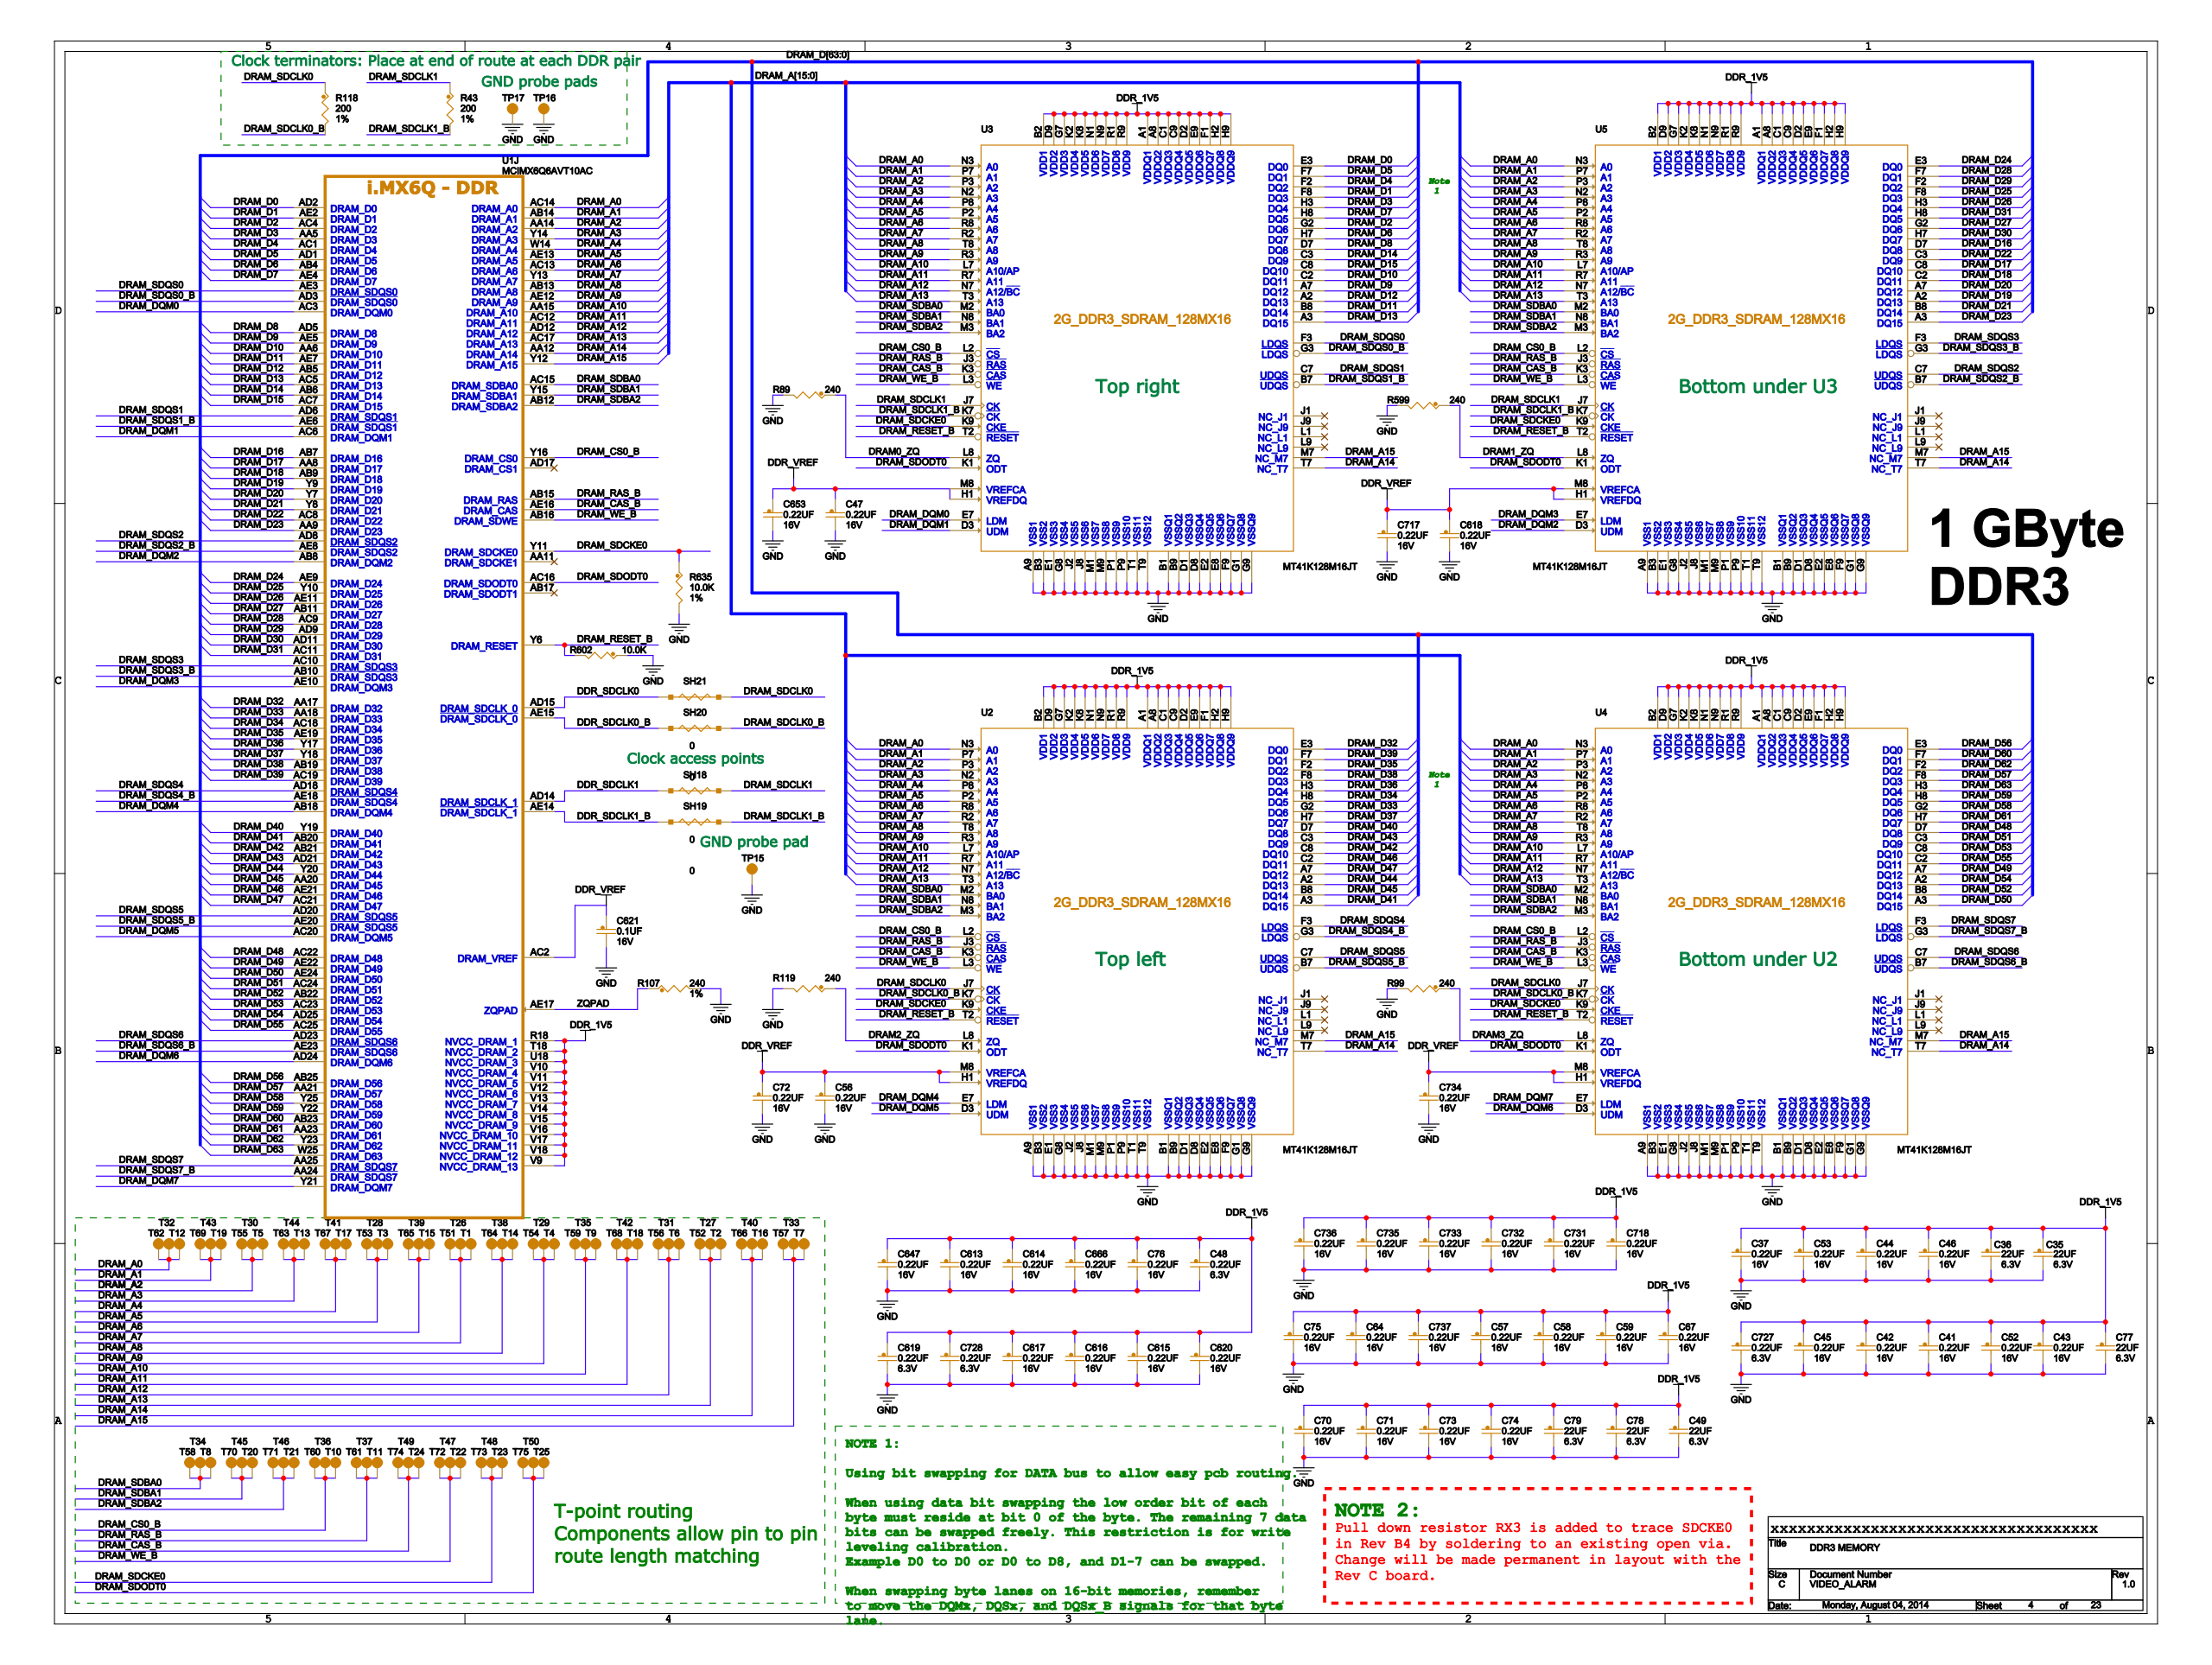Circuit board | Cadence Allegro | 994 parts | 728 nets | one sheet of the schematic
Parts on this sheet (reference | value | footprint):
C35 | 22UF | 0805_CC
C36 | 22UF | 0805_CC
C37 | 0.22UF | 0402_CC
C41 | 0.22UF | 0402_CC
C42 | 0.22UF | 0402_CC
C43 | 0.22UF | 0402_CC
C44 | 0.22UF | 0402_CC
C45 | 0.22UF | 0402_CC
C46 | 0.22UF | 0402_CC
C47 | 0.22UF | 0402_CC
C48 | 0.22UF | 0201_CC
C49 | 22UF | 0805_CC
C52 | 0.22UF | 0402_CC
C53 | 0.22UF | 0402_CC
C56 | 0.22UF | 0402_CC
C57 | 0.22UF | 0402_CC
C58 | 0.22UF | 0402_CC
C59 | 0.22UF | 0402_CC
C64 | 0.22UF | 0402_CC
C67 | 0.22UF | 0402_CC
C70 | 0.22UF | 0402_CC
C71 | 0.22UF | 0402_CC
C72 | 0.22UF | 0402_CC
C73 | 0.22UF | 0402_CC
C74 | 0.22UF | 0402_CC
C75 | 0.22UF | 0402_CC
C76 | 0.22UF | 0402_CC
C77 | 22UF | 0805_CC
C78 | 22UF | 0805_CC
C79 | 22UF | 0805_CC
C613 | 0.22UF | 0402_CC
C614 | 0.22UF | 0402_CC
C615 | 0.22UF | 0402_CC
C616 | 0.22UF | 0402_CC
C617 | 0.22UF | 0402_CC
C618 | 0.22UF | 0402_CC
C619 | 0.22UF | 0201_CC
C620 | 0.22UF | 0402_CC
C621 | 0.1UF | 0402_CC
C647 | 0.22UF | 0402_CC
C653 | 0.22UF | 0402_CC
C666 | 0.22UF | 0402_CC
C717 | 0.22UF | 0402_CC
C718 | 0.22UF | 0402_CC
C727 | 0.22UF | 0201_CC
C728 | 0.22UF | 0201_CC
C731 | 0.22UF | 0402_CC
C732 | 0.22UF | 0402_CC
C733 | 0.22UF | 0402_CC
C734 | 0.22UF | 0402_CC
C735 | 0.22UF | 0402_CC
C736 | 0.22UF | 0402_CC
C737 | 0.22UF | 0402_CC
J8 | 10029449-001RLF | HDMI
R43 | 200 | 0402_CC
R89 | 240 | 0402_CC
R99 | 240 | 0402_CC
R107 | 240 | 0402_CC
R118 | 200 | 0402_CC
R119 | 240 | 0402_CC
R599 | 240 | 0402_CC
R602 | 10.0K | 0402_CC
R635 | 10.0K | 0402_CC
SH18 | 0 | SH0201_CC
SH19 | 0 | SH0201_CC
SH20 | 0 | SH0201_CC
SH21 | 0 | SH0201_CC
T1 | TPAD_015 | TPAD_015
T2 | TPAD_015 | TPAD_015
T3 | TPAD_015 | TPAD_015
T4 | TPAD_015 | TPAD_015
T5 | TPAD_015 | TPAD_015
T6 | TPAD_015 | TPAD_015
T7 | TPAD_015 | TPAD_015
T8 | TPAD_015 | TPAD_015
T9 | TPAD_015 | TPAD_015
T10 | TPAD_015 | TPAD_015
T11 | TPAD_015 | TPAD_015
T12 | TPAD_015 | TPAD_015
T13 | TPAD_015 | TPAD_015
T14 | TPAD_015 | TPAD_015
T15 | TPAD_015 | TPAD_015
T16 | TPAD_015 | TPAD_015
T17 | TPAD_015 | TPAD_015
T18 | TPAD_015 | TPAD_015
T19 | TPAD_015 | TPAD_015
T20 | TPAD_015 | TPAD_015
T21 | TPAD_015 | TPAD_015
T22 | TPAD_015 | TPAD_015
T23 | TPAD_015 | TPAD_015
T24 | TPAD_015 | TPAD_015
T25 | TPAD_015 | TPAD_015
T26 | TPAD_015 | TPAD_015
T27 | TPAD_015 | TPAD_015
T28 | TPAD_015 | TPAD_015
T29 | TPAD_015 | TPAD_015
T30 | TPAD_015 | TPAD_015
T31 | TPAD_015 | TPAD_015
T32 | TPAD_015 | TPAD_015
T33 | TPAD_015 | TPAD_015
T34 | TPAD_015 | TPAD_015
T35 | TPAD_015 | TPAD_015
T36 | TPAD_015 | TPAD_015
T37 | TPAD_015 | TPAD_015
T38 | TPAD_015 | TPAD_015
T39 | TPAD_015 | TPAD_015
T40 | TPAD_015 | TPAD_015
T41 | TPAD_015 | TPAD_015
T42 | TPAD_015 | TPAD_015
T43 | TPAD_015 | TPAD_015
T44 | TPAD_015 | TPAD_015
T45 | TPAD_015 | TPAD_015
T46 | TPAD_015 | TPAD_015
T47 | TPAD_015 | TPAD_015
T48 | TPAD_015 | TPAD_015
T49 | TPAD_015 | TPAD_015
T50 | TPAD_015 | TPAD_015
T51 | TPAD_015 | TPAD_015
T52 | TPAD_015 | TPAD_015
T53 | TPAD_015 | TPAD_015
T54 | TPAD_015 | TPAD_015
T55 | TPAD_015 | TPAD_015
T56 | TPAD_015 | TPAD_015
T57 | TPAD_015 | TPAD_015
T58 | TPAD_015 | TPAD_015
T59 | TPAD_015 | TPAD_015
T60 | TPAD_015 | TPAD_015
T61 | TPAD_015 | TPAD_015
T62 | TPAD_015 | TPAD_015
T63 | TPAD_015 | TPAD_015
T64 | TPAD_015 | TPAD_015
T65 | TPAD_015 | TPAD_015
T66 | TPAD_015 | TPAD_015
T67 | TPAD_015 | TPAD_015
T68 | TPAD_015 | TPAD_015
T69 | TPAD_015 | TPAD_015
T70 | TPAD_015 | TPAD_015
T71 | TPAD_015 | TPAD_015
T72 | TPAD_015 | TPAD_015
T73 | TPAD_015 | TPAD_015
T74 | TPAD_015 | TPAD_015
T75 | TPAD_015 | TPAD_015
TP15 | TPAD_020 | TPAD_020
TP16 | TPAD_020 | TPAD_020
TP17 | TPAD_020 | TPAD_020
U1 | MCIMX6Q6AVT10AC | BGA624_0P8_21X21
U2 | MT41K128M16JT | BGA96_0P8_8P15X14P15
U3 | MT41K128M16JT | BGA96_0P8_8P15X14P15
U4 | MT41K128M16JT | BGA96_0P8_8P15X14P15
U5 | MT41K128M16JT | BGA96_0P8_8P15X14P15
Nets of these parts (net: part-pin ...):
GND: C35-2 C36-2 C37-2 C41-2 C42-2 C43-2 C44-2 C45-2 C46-2 C47-2 C48-2 C49-2 C52-2 C53-2 C56-2 C57-2 C58-2 C59-2 C64-2 C67-2 C70-2 C71-2 C72-2 C73-2 C74-2 C75-2 C76-2 C77-2 C78-2 C79-2 C613-2 C614-2 C615-2 C616-2 C617-2 C618-2 C619-2 C620-2 C621-2 C647-2 C653-2 C666-2 C717-2 C718-2 C727-2 C728-2 C731-2 C732-2 C733-2 C734-2 C735-2 C736-2 C737-2 R89-2 R99-2 R107-2 R119-2 R599-2 R602-1 R635-2 TP15-1 TP16-1 TP17-1 J8-2 J8-5 U1-A4 U1-A5 U1-A8 U1-A13 U1-B4 U1-C1 U1-D3 U1-D8 U1-E7 U1-F7 U1-F8 U1-G3 U1-H8 U1-J2 U1-J8 U1-K8 U1-L2 U1-L8 U1-M8 U1-N8 U1-P8 U1-R8 U1-T8 U1-T11 U1-T12 U1-T15 U1-T17 U1-T19 U2-A9 U2-B1 U2-B3 U2-B9 U2-D1 U2-D8 U2-E1 U2-E2 U2-E8 U2-F9 U2-G1 U2-G8 U2-G9 U2-J2 U2-J8 U2-M1 U2-M9 U2-P1 U2-P9 U2-T1 U2-T9 U3-A9 U3-B1 U3-B3 U3-B9 U3-D1 U3-D8 U3-E1 U3-E2 U3-E8 U3-F9 U3-G1 U3-G8 U3-G9 U3-J2 U3-J8 U3-M1 U3-M9 U3-P1 U3-P9 U3-T1 U3-T9 U4-A9 U4-B1 U4-B3 U4-B9 U4-D1 U4-D8 U4-E1 U4-E2 U4-E8 U4-F9 U4-G1 U4-G8 U4-G9 U4-J2 U4-J8 U4-M1 U4-M9 U4-P1 U4-P9 U4-T1 U4-T9 U5-A9 U5-B1 U5-B3 U5-B9 U5-D1 U5-D8 U5-E1 U5-E2 U5-E8 U5-F9 U5-G1 U5-G8 U5-G9 U5-J2 U5-J8 U5-M1 U5-M9 U5-P1 U5-P9 U5-T1 U5-T9
DDR_1V5: C35-1 C36-1 C37-1 C41-1 C42-1 C43-1 C44-1 C45-1 C46-1 C48-1 C49-1 C52-1 C53-1 C57-1 C58-1 C59-1 C64-1 C67-1 C70-1 C71-1 C73-1 C74-1 C75-1 C76-1 C77-1 C78-1 C79-1 C613-1 C614-1 C615-1 C616-1 C617-1 C619-1 C620-1 C647-1 C666-1 C718-1 C727-1 C728-1 C731-1 C732-1 C733-1 C735-1 C736-1 C737-1 U1-R18 U1-T18 U1-U18 U1-V9 U1-V10 U1-V11 U1-V12 U1-V13 U1-V14 U1-V15 U1-V16 U1-V17 U1-V18 U2-A1 U2-A8 U2-B2 U2-C1 U2-C9 U2-D2 U2-D9 U2-E9 U2-F1 U2-G7 U2-H2 U2-H9 U2-K2 U2-K8 U2-N1 U2-N9 U2-R1 U2-R9 U3-A1 U3-A8 U3-B2 U3-C1 U3-C9 U3-D2 U3-D9 U3-E9 U3-F1 U3-G7 U3-H2 U3-H9 U3-K2 U3-K8 U3-N1 U3-N9 U3-R1 U3-R9 U4-A1 U4-A8 U4-B2 U4-C1 U4-C9 U4-D2 U4-D9 U4-E9 U4-F1 U4-G7 U4-H2 U4-H9 U4-K2 U4-K8 U4-N1 U4-N9 U4-R1 U4-R9 U5-A1 U5-A8 U5-B2 U5-C1 U5-C9 U5-D2 U5-D9 U5-E9 U5-F1 U5-G7 U5-H2 U5-H9 U5-K2 U5-K8 U5-N1 U5-N9 U5-R1 U5-R9
DDR_VREF: C47-1 C56-1 C72-1 C618-1 C621-1 C653-1 C717-1 C734-1 U1-AC2 U2-H1 U2-M8 U3-H1 U3-M8 U4-H1 U4-M8 U5-H1 U5-M8
DDR_SDCLK0: SH21-1 U1-AD15
DRAM_SDCLK0: R118-1 SH21-2 U2-J7 U4-J7
DDR_SDCLK0_B: SH20-1 U1-AE15
DRAM_SDCLK0_B: R118-2 SH20-2 U2-K7 U4-K7
DDR_SDCLK1_B: SH19-1 U1-AE14
DRAM_SDCLK1_B: R43-2 SH19-2 U3-K7 U5-K7
DDR_SDCLK1: SH18-1 U1-AD14
DRAM_SDCLK1: R43-1 SH18-2 U3-J7 U5-J7
DRAM_A0: T12-1 T32-1 T62-1 U1-AC14 U2-N3 U3-N3 U4-N3 U5-N3
DRAM_A1: T19-1 T43-1 T69-1 U1-AB14 U2-P7 U3-P7 U4-P7 U5-P7
DRAM_A10: T9-1 T35-1 T59-1 U1-AA15 U2-L7 U3-L7 U4-L7 U5-L7
DRAM_A11: T18-1 T42-1 T68-1 U1-AC12 U2-R7 U3-R7 U4-R7 U5-R7
DRAM_A12: T6-1 T31-1 T56-1 U1-AD12 U2-N7 U3-N7 U4-N7 U5-N7
DRAM_A13: T2-1 T27-1 T52-1 U1-AC17 U2-T3 U3-T3 U4-T3 U5-T3
DRAM_A2: T5-1 T30-1 T55-1 U1-AA14 U2-P3 U3-P3 U4-P3 U5-P3
DRAM_A3: T13-1 T44-1 T63-1 U1-Y14 U2-N2 U3-N2 U4-N2 U5-N2
DRAM_A4: T17-1 T41-1 T67-1 U1-W14 U2-P8 U3-P8 U4-P8 U5-P8
DRAM_A5: T3-1 T28-1 T53-1 U1-AE13 U2-P2 U3-P2 U4-P2 U5-P2
DRAM_A6: T15-1 T39-1 T65-1 U1-AC13 U2-R8 U3-R8 U4-R8 U5-R8
DRAM_A7: T1-1 T26-1 T51-1 U1-Y13 U2-R2 U3-R2 U4-R2 U5-R2
DRAM_A8: T14-1 T38-1 T64-1 U1-AB13 U2-T8 U3-T8 U4-T8 U5-T8
DRAM_A9: T4-1 T29-1 T54-1 U1-AE12 U2-R3 U3-R3 U4-R3 U5-R3
DRAM_SDBA0: T8-1 T34-1 T58-1 U1-AC15 U2-M2 U3-M2 U4-M2 U5-M2
DRAM_SDBA1: T20-1 T45-1 T70-1 U1-Y15 U2-N8 U3-N8 U4-N8 U5-N8
DRAM_SDBA2: T21-1 T46-1 T71-1 U1-AB12 U2-M3 U3-M3 U4-M3 U5-M3
DRAM_SDCKE0: R635-1 T23-1 T48-1 T73-1 U1-Y11 U2-K9 U3-K9 U4-K9 U5-K9
DRAM_CAS_B: T24-1 T49-1 T74-1 U1-AE16 U2-K3 U3-K3 U4-K3 U5-K3
DRAM_CS0_B: T10-1 T36-1 T60-1 U1-Y16 U2-L2 U3-L2 U4-L2 U5-L2
DRAM_D24: U1-AE9 U5-E3
DRAM_D28: U1-AC9 U5-F7
DRAM_D17: U1-AA8 U5-C8
DRAM_D18: U1-AB9 U5-C2
DRAM_D20: U1-Y7 U5-A7
DRAM_D19: U1-Y9 U5-A2
DRAM_D21: U1-Y8 U5-B8
DRAM_D23: U1-AA9 U5-A3
DRAM_D29: U1-AD9 U5-F2
DRAM_D25: U1-Y10 U5-F8
DRAM_D26: U1-AE11 U5-H3
DRAM_D31: U1-AC11 U5-H8
DRAM_D27: U1-AB11 U5-G2
DRAM_D30: U1-AD11 U5-H7
DRAM_D16: U1-AB7 U5-D7
DRAM_D22: U1-AC8 U5-C3
DRAM_DQM3: U1-AE10 U5-E7
DRAM_SDQS3: U1-AC10 U5-F3
DRAM_SDQS3_B: U1-AB10 U5-G3
DRAM_A15: T7-1 T33-1 T57-1 U1-Y12 U2-M7 U3-M7 U4-M7 U5-M7
DRAM_A14: T16-1 T40-1 T66-1 U1-AA12 U2-T7 U3-T7 U4-T7 U5-T7
DRAM_SDODT0: T25-1 T50-1 T75-1 U1-AC16 U2-K1 U3-K1 U4-K1 U5-K1
DRAM_RAS_B: T11-1 T37-1 T61-1 U1-AB15 U2-J3 U3-J3 U4-J3 U5-J3
DRAM_RESET_B: R602-2 U1-Y6 U2-T2 U3-T2 U4-T2 U5-T2
DRAM_DQM2: U1-AB8 U5-D3
DRAM_SDQS2: U1-AD8 U5-C7
DRAM_SDQS2_B: U1-AE8 U5-B7
DRAM_WE_B: T22-1 T47-1 T72-1 U1-AB16 U2-L3 U3-L3 U4-L3 U5-L3
DRAM1_ZQ: R599-1 U5-L8
DRAM_D56: U1-AB25 U4-E3
DRAM_D60: U1-AB23 U4-F7
DRAM_D53: U1-AC23 U4-C8
DRAM_D55: U1-AC25 U4-C2
DRAM_D49: U1-AE22 U4-A7
DRAM_D54: U1-AD25 U4-A2
DRAM_D52: U1-AB22 U4-B8
DRAM_D50: U1-AE24 U4-A3
DRAM_D62: U1-Y23 U4-F2
DRAM_D57: U1-AA21 U4-F8
DRAM_D63: U1-W25 U4-H3
DRAM_D59: U1-Y22 U4-H8
DRAM_D58: U1-Y25 U4-G2
DRAM_D61: U1-AA23 U4-H7
DRAM_D48: U1-AC22 U4-D7
DRAM_D51: U1-AC24 U4-C3
DRAM_DQM7: U1-Y21 U4-E7
DRAM_SDQS7: U1-AA25 U4-F3
DRAM_SDQS7_B: U1-AA24 U4-G3
DRAM_DQM6: U1-AD24 U4-D3
DRAM_SDQS6: U1-AD23 U4-C7
DRAM_SDQS6_B: U1-AE23 U4-B7
DRAM3_ZQ: R99-1 U4-L8
DRAM_D0: U1-AD2 U3-E3
DRAM_D5: U1-AD1 U3-F7
DRAM_D15: U1-AC7 U3-C8
DRAM_D10: U1-AA6 U3-C2
DRAM_D9: U1-AE5 U3-A7
DRAM_D12: U1-AB5 U3-A2
DRAM_D11: U1-AE7 U3-B8
DRAM_D13: U1-AC5 U3-A3
DRAM_D4: U1-AC1 U3-F2
DRAM_D1: U1-AE2 U3-F8
DRAM_D3: U1-AA5 U3-H3
DRAM_D7: U1-AE4 U3-H8
DRAM_D2: U1-AC4 U3-G2
DRAM_D6: U1-AB4 U3-H7
DRAM_D8: U1-AD5 U3-D7
DRAM_D14: U1-AB6 U3-C3
DRAM_DQM0: U1-AC3 U3-E7
DRAM_SDQS0: U1-AE3 U3-F3
DRAM_SDQS0_B: U1-AD3 U3-G3
DRAM_DQM1: U1-AC6 U3-D3
DRAM_SDQS1: U1-AD6 U3-C7
DRAM_SDQS1_B: U1-AE6 U3-B7
DRAM0_ZQ: R89-1 U3-L8
DRAM_D32: U1-AA17 U2-E3
DRAM_D39: U1-AC19 U2-F7
DRAM_D42: U1-AB21 U2-C8
DRAM_D46: U1-AE21 U2-C2
DRAM_D47: U1-AC21 U2-A7
DRAM_D44: U1-Y20 U2-A2
DRAM_D45: U1-AA20 U2-B8
DRAM_D41: U1-AB20 U2-A3
DRAM_D35: U1-AE19 U2-F2
DRAM_D38: U1-AB19 U2-F8
DRAM_D36: U1-Y17 U2-H3
DRAM_D34: U1-AC18 U2-H8
DRAM_D33: U1-AA18 U2-G2
DRAM_D37: U1-Y18 U2-H7
DRAM_D40: U1-Y19 U2-D7
DRAM_D43: U1-AD21 U2-C3
DRAM_DQM4: U1-AB18 U2-E7
DRAM_SDQS4: U1-AD18 U2-F3
DRAM_SDQS4_B: U1-AE18 U2-G3
DRAM_DQM5: U1-AC20 U2-D3
DRAM_SDQS5: U1-AD20 U2-C7
DRAM_SDQS5_B: U1-AE20 U2-B7
DRAM2_ZQ: R119-1 U2-L8
ZQPAD: R107-1 U1-AE17